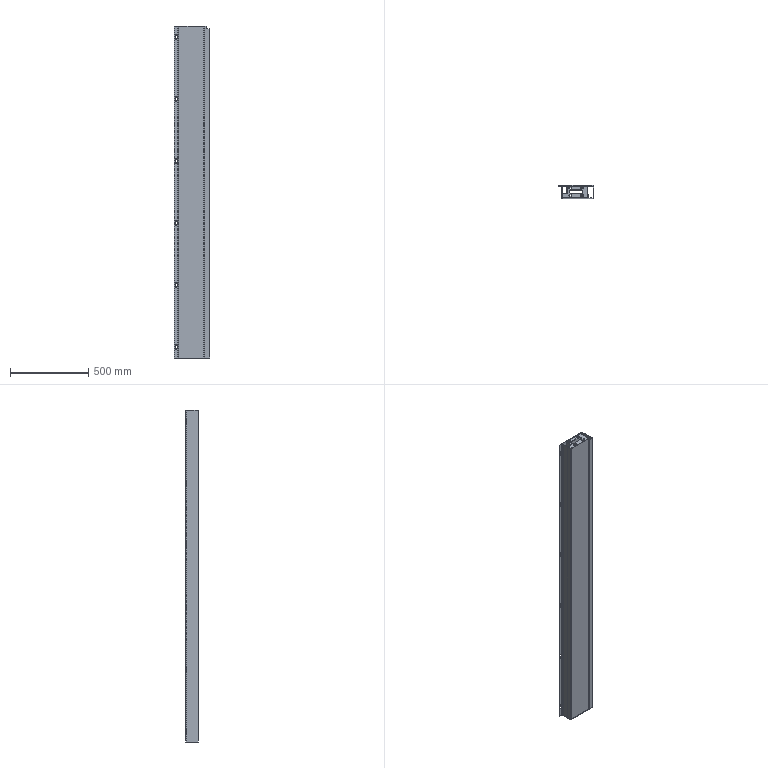Part | SolidWorks | features Fillet 6, ICE 5, Extrusion 1, MirrorSolid 1 | 5 solids | 154 faces | box 225 x 80 x 2116 mm | volume 3306402 mm3 | plane 88 | cylinder 66 | commonest cylinder face diameters 10 x24 9 x18 2 x9 6 x8 25 x6 8 x1